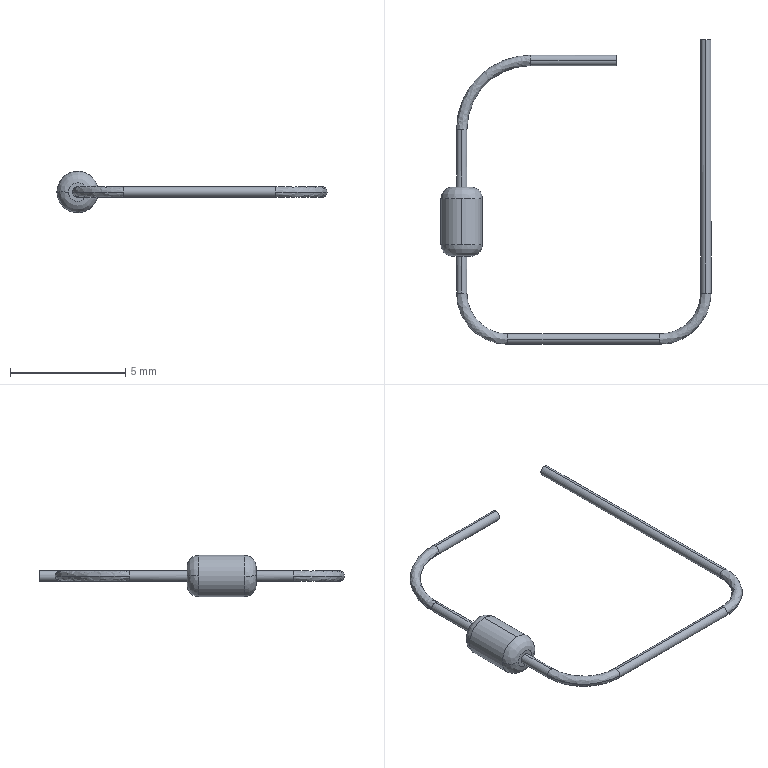Part | STEP file | TQ-DD-1105-THNTC Thermistor1010_デフォルト | 1 solid | 26 faces | box 11.725 x 13.225 x 1.8 mm | volume 12.894 mm3 | cylinder 12 | spline 10 | plane 4 | commonest cylinder face diameters 0.45 x10 1.8 x2
STEP:
#1=CARTESIAN_POINT('',(10.825,-3.1,0.));
#2=VERTEX_POINT('',#1);
#3=CARTESIAN_POINT('',(10.6,-3.1,-0.225));
#4=VERTEX_POINT('',#3);
#5=CARTESIAN_POINT('',(10.6,-3.1,0.));
#6=DIRECTION('',(0.,1.,0.));
#7=DIRECTION('',(0.,0.,1.));
#8=AXIS2_PLACEMENT_3D('',#5,#6,#7);
#9=CIRCLE('',#8,0.225);
#10=EDGE_CURVE('',#2,#4,#9,.T.);
#11=ORIENTED_EDGE('',*,*,#10,.T.);
#12=CARTESIAN_POINT('',(10.6,7.9,-0.225));
#13=VERTEX_POINT('',#12);
#14=CARTESIAN_POINT('',(10.6,2.4,-0.225));
#15=DIRECTION('',(0.,1.,0.));
#16=VECTOR('',#15,1000.);
#17=LINE('',#14,#16);
#18=EDGE_CURVE('',#4,#13,#17,.T.);
#19=ORIENTED_EDGE('',*,*,#18,.T.);
#20=CARTESIAN_POINT('',(10.6,7.9,0.225));
#21=VERTEX_POINT('',#20);
#22=CARTESIAN_POINT('',(10.6,7.9,0.));
#23=DIRECTION('',(0.,-1.,0.));
#24=DIRECTION('',(0.,0.,1.));
#25=AXIS2_PLACEMENT_3D('',#22,#23,#24);
#26=CIRCLE('',#25,0.225);
#27=EDGE_CURVE('',#13,#21,#26,.T.);
#28=ORIENTED_EDGE('',*,*,#27,.T.);
#29=CARTESIAN_POINT('',(10.6,-3.1,0.225));
#30=VERTEX_POINT('',#29);
#31=CARTESIAN_POINT('',(10.6,2.4,0.225));
#32=DIRECTION('',(0.,1.,0.));
#33=VECTOR('',#32,1000.);
#34=LINE('',#31,#33);
#35=EDGE_CURVE('',#30,#21,#34,.T.);
#36=ORIENTED_EDGE('',*,*,#35,.F.);
#37=CARTESIAN_POINT('',(10.6,-3.1,0.));
#38=DIRECTION('',(0.,1.,0.));
#39=DIRECTION('',(0.,0.,1.));
#40=AXIS2_PLACEMENT_3D('',#37,#38,#39);
#41=CIRCLE('',#40,0.225);
#42=EDGE_CURVE('',#30,#2,#41,.T.);
#43=ORIENTED_EDGE('',*,*,#42,.T.);
#44=EDGE_LOOP('',(#11,#19,#28,#36,#43));
#45=FACE_OUTER_BOUND('',#44,.T.);
#46=CARTESIAN_POINT('',(10.6,2.4,0.));
#47=DIRECTION('',(0.,1.,0.));
#48=DIRECTION('',(0.,0.,1.));
#49=AXIS2_PLACEMENT_3D('',#46,#47,#48);
#50=CYLINDRICAL_SURFACE('',#49,0.225);
#51=ADVANCED_FACE('',(#45),#50,.T.);
#52=CARTESIAN_POINT('',(8.6,-5.1,-0.225));
#53=VERTEX_POINT('',#52);
#54=CARTESIAN_POINT('',(8.6,-4.875,0.));
#55=VERTEX_POINT('',#54);
#56=CARTESIAN_POINT('',(8.6,-5.1,0.));
#57=DIRECTION('',(1.,0.,0.));
#58=DIRECTION('',(0.,-1.,0.));
#59=AXIS2_PLACEMENT_3D('',#56,#57,#58);
#60=CIRCLE('',#59,0.225);
#61=EDGE_CURVE('',#53,#55,#60,.T.);
#62=ORIENTED_EDGE('',*,*,#61,.T.);
#63=CARTESIAN_POINT('',(10.375,-3.1,0.));
#64=VERTEX_POINT('',#63);
#65=CARTESIAN_POINT('',(8.6,-3.1,0.));
#66=DIRECTION('',(0.,0.,1.));
#67=DIRECTION('',(0.,-1.,0.));
#68=AXIS2_PLACEMENT_3D('',#65,#66,#67);
#69=CIRCLE('',#68,1.775);
#70=EDGE_CURVE('',#55,#64,#69,.T.);
#71=ORIENTED_EDGE('',*,*,#70,.T.);
#72=CARTESIAN_POINT('',(10.6,-3.1,0.));
#73=DIRECTION('',(0.,1.,0.));
#74=DIRECTION('',(0.,0.,1.));
#75=AXIS2_PLACEMENT_3D('',#72,#73,#74);
#76=CIRCLE('',#75,0.225);
#77=EDGE_CURVE('',#4,#64,#76,.T.);
#78=ORIENTED_EDGE('',*,*,#77,.F.);
#79=ORIENTED_EDGE('',*,*,#10,.F.);
#80=CARTESIAN_POINT('',(8.6,-5.325,0.));
#81=VERTEX_POINT('',#80);
#82=CARTESIAN_POINT('',(8.6,-3.1,0.));
#83=DIRECTION('',(0.,0.,1.));
#84=DIRECTION('',(0.,-1.,0.));
#85=AXIS2_PLACEMENT_3D('',#82,#83,#84);
#86=CIRCLE('',#85,2.225);
#87=EDGE_CURVE('',#81,#2,#86,.T.);
#88=ORIENTED_EDGE('',*,*,#87,.F.);
#89=CARTESIAN_POINT('',(8.6,-5.1,0.));
#90=DIRECTION('',(1.,0.,0.));
#91=DIRECTION('',(0.,-1.,0.));
#92=AXIS2_PLACEMENT_3D('',#89,#90,#91);
#93=CIRCLE('',#92,0.225);
#94=EDGE_CURVE('',#81,#53,#93,.T.);
#95=ORIENTED_EDGE('',*,*,#94,.T.);
#96=EDGE_LOOP('',(#62,#71,#78,#79,#88,#95));
#97=FACE_OUTER_BOUND('',#96,.T.);
#98=CARTESIAN_POINT('',(8.6,-5.325,0.));
#99=CARTESIAN_POINT('',(9.903,-5.325,0.));
#100=CARTESIAN_POINT('',(10.825,-4.403,0.));
#101=CARTESIAN_POINT('',(10.825,-3.1,0.));
#102=CARTESIAN_POINT('',(8.6,-5.325,-0.45));
#103=CARTESIAN_POINT('',(9.903,-5.325,-0.45));
#104=CARTESIAN_POINT('',(10.825,-4.403,-0.45));
#105=CARTESIAN_POINT('',(10.825,-3.1,-0.45));
#106=CARTESIAN_POINT('',(8.6,-4.875,-0.45));
#107=CARTESIAN_POINT('',(9.64,-4.875,-0.45));
#108=CARTESIAN_POINT('',(10.375,-4.14,-0.45));
#109=CARTESIAN_POINT('',(10.375,-3.1,-0.45));
#110=CARTESIAN_POINT('',(8.6,-4.875,0.));
#111=CARTESIAN_POINT('',(9.64,-4.875,0.));
#112=CARTESIAN_POINT('',(10.375,-4.14,0.));
#113=CARTESIAN_POINT('',(10.375,-3.1,0.));
#114=(BOUNDED_SURFACE()B_SPLINE_SURFACE(3,3,((#98,#99,#100,#101),(#102,#103,#104,#105),(#106,#107,#108,#109),(#110,#111,#112,#113)),.UNSPECIFIED.,.F.,.F.,.F.)B_SPLINE_SURFACE_WITH_KNOTS((4,4),(4,4),(0.,1.),(0.,1.),.UNSPECIFIED.)GEOMETRIC_REPRESENTATION_ITEM()RATIONAL_B_SPLINE_SURFACE(((1.,0.8047,0.8047,1.),(0.3333,0.2682,0.2682,0.3333),(0.3333,0.2682,0.2682,0.3333),(1.,0.8047,0.8047,1.)))REPRESENTATION_ITEM('')SURFACE());
#115=ADVANCED_FACE('',(#97),#114,.T.);
#116=CARTESIAN_POINT('',(2.,-4.875,0.));
#117=VERTEX_POINT('',#116);
#118=CARTESIAN_POINT('',(2.,-5.1,0.225));
#119=VERTEX_POINT('',#118);
#120=CARTESIAN_POINT('',(2.,-5.1,0.));
#121=DIRECTION('',(1.,0.,0.));
#122=DIRECTION('',(0.,0.,-1.));
#123=AXIS2_PLACEMENT_3D('',#120,#121,#122);
#124=CIRCLE('',#123,0.225);
#125=EDGE_CURVE('',#117,#119,#124,.T.);
#126=ORIENTED_EDGE('',*,*,#125,.T.);
#127=CARTESIAN_POINT('',(8.6,-5.1,0.225));
#128=VERTEX_POINT('',#127);
#129=CARTESIAN_POINT('',(5.3,-5.1,0.225));
#130=DIRECTION('',(1.,0.,0.));
#131=VECTOR('',#130,1000.);
#132=LINE('',#129,#131);
#133=EDGE_CURVE('',#119,#128,#132,.T.);
#134=ORIENTED_EDGE('',*,*,#133,.T.);
#135=CARTESIAN_POINT('',(8.6,-5.1,0.));
#136=DIRECTION('',(1.,0.,0.));
#137=DIRECTION('',(0.,-1.,0.));
#138=AXIS2_PLACEMENT_3D('',#135,#136,#137);
#139=CIRCLE('',#138,0.225);
#140=EDGE_CURVE('',#55,#128,#139,.T.);
#141=ORIENTED_EDGE('',*,*,#140,.F.);
#142=ORIENTED_EDGE('',*,*,#61,.F.);
#143=CARTESIAN_POINT('',(2.,-5.1,-0.225));
#144=VERTEX_POINT('',#143);
#145=CARTESIAN_POINT('',(5.3,-5.1,-0.225));
#146=DIRECTION('',(1.,0.,0.));
#147=VECTOR('',#146,1000.);
#148=LINE('',#145,#147);
#149=EDGE_CURVE('',#144,#53,#148,.T.);
#150=ORIENTED_EDGE('',*,*,#149,.F.);
#151=CARTESIAN_POINT('',(2.,-5.1,0.));
#152=DIRECTION('',(1.,0.,0.));
#153=DIRECTION('',(0.,0.,-1.));
#154=AXIS2_PLACEMENT_3D('',#151,#152,#153);
#155=CIRCLE('',#154,0.225);
#156=EDGE_CURVE('',#144,#117,#155,.T.);
#157=ORIENTED_EDGE('',*,*,#156,.T.);
#158=EDGE_LOOP('',(#126,#134,#141,#142,#150,#157));
#159=FACE_OUTER_BOUND('',#158,.T.);
#160=CARTESIAN_POINT('',(5.3,-5.1,0.));
#161=DIRECTION('',(1.,0.,0.));
#162=DIRECTION('',(0.,0.,-1.));
#163=AXIS2_PLACEMENT_3D('',#160,#161,#162);
#164=CYLINDRICAL_SURFACE('',#163,0.225);
#165=ADVANCED_FACE('',(#159),#164,.T.);
#166=CARTESIAN_POINT('',(0.,-3.1,-0.225));
#167=VERTEX_POINT('',#166);
#168=CARTESIAN_POINT('',(0.225,-3.1,0.));
#169=VERTEX_POINT('',#168);
#170=CARTESIAN_POINT('',(0.,-3.1,0.));
#171=DIRECTION('',(0.,-1.,0.));
#172=DIRECTION('',(-1.,0.,0.));
#173=AXIS2_PLACEMENT_3D('',#170,#171,#172);
#174=CIRCLE('',#173,0.225);
#175=EDGE_CURVE('',#167,#169,#174,.T.);
#176=ORIENTED_EDGE('',*,*,#175,.T.);
#177=CARTESIAN_POINT('',(2.,-3.1,0.));
#178=DIRECTION('',(0.,0.,1.));
#179=DIRECTION('',(-1.,0.,0.));
#180=AXIS2_PLACEMENT_3D('',#177,#178,#179);
#181=CIRCLE('',#180,1.775);
#182=EDGE_CURVE('',#169,#117,#181,.T.);
#183=ORIENTED_EDGE('',*,*,#182,.T.);
#184=ORIENTED_EDGE('',*,*,#156,.F.);
#185=CARTESIAN_POINT('',(2.,-5.325,0.));
#186=VERTEX_POINT('',#185);
#187=CARTESIAN_POINT('',(2.,-5.1,0.));
#188=DIRECTION('',(1.,0.,0.));
#189=DIRECTION('',(0.,0.,-1.));
#190=AXIS2_PLACEMENT_3D('',#187,#188,#189);
#191=CIRCLE('',#190,0.225);
#192=EDGE_CURVE('',#186,#144,#191,.T.);
#193=ORIENTED_EDGE('',*,*,#192,.F.);
#194=CARTESIAN_POINT('',(-0.225,-3.1,0.));
#195=VERTEX_POINT('',#194);
#196=CARTESIAN_POINT('',(2.,-3.1,0.));
#197=DIRECTION('',(0.,0.,1.));
#198=DIRECTION('',(-1.,0.,0.));
#199=AXIS2_PLACEMENT_3D('',#196,#197,#198);
#200=CIRCLE('',#199,2.225);
#201=EDGE_CURVE('',#195,#186,#200,.T.);
#202=ORIENTED_EDGE('',*,*,#201,.F.);
#203=CARTESIAN_POINT('',(0.,-3.1,0.));
#204=DIRECTION('',(0.,-1.,0.));
#205=DIRECTION('',(-1.,0.,0.));
#206=AXIS2_PLACEMENT_3D('',#203,#204,#205);
#207=CIRCLE('',#206,0.225);
#208=EDGE_CURVE('',#195,#167,#207,.T.);
#209=ORIENTED_EDGE('',*,*,#208,.T.);
#210=EDGE_LOOP('',(#176,#183,#184,#193,#202,#209));
#211=FACE_OUTER_BOUND('',#210,.T.);
#212=CARTESIAN_POINT('',(-0.225,-3.1,0.));
#213=CARTESIAN_POINT('',(-0.225,-4.403,0.));
#214=CARTESIAN_POINT('',(0.6966,-5.325,0.));
#215=CARTESIAN_POINT('',(2.,-5.325,0.));
#216=CARTESIAN_POINT('',(-0.225,-3.1,-0.45));
#217=CARTESIAN_POINT('',(-0.225,-4.403,-0.45));
#218=CARTESIAN_POINT('',(0.6966,-5.325,-0.45));
#219=CARTESIAN_POINT('',(2.,-5.325,-0.45));
#220=CARTESIAN_POINT('',(0.225,-3.1,-0.45));
#221=CARTESIAN_POINT('',(0.225,-4.14,-0.45));
#222=CARTESIAN_POINT('',(0.9602,-4.875,-0.45));
#223=CARTESIAN_POINT('',(2.,-4.875,-0.45));
#224=CARTESIAN_POINT('',(0.225,-3.1,0.));
#225=CARTESIAN_POINT('',(0.225,-4.14,0.));
#226=CARTESIAN_POINT('',(0.9602,-4.875,0.));
#227=CARTESIAN_POINT('',(2.,-4.875,0.));
#228=(BOUNDED_SURFACE()B_SPLINE_SURFACE(3,3,((#212,#213,#214,#215),(#216,#217,#218,#219),(#220,#221,#222,#223),(#224,#225,#226,#227)),.UNSPECIFIED.,.F.,.F.,.F.)B_SPLINE_SURFACE_WITH_KNOTS((4,4),(4,4),(0.,1.),(0.,1.),.UNSPECIFIED.)GEOMETRIC_REPRESENTATION_ITEM()RATIONAL_B_SPLINE_SURFACE(((1.,0.8047,0.8047,1.),(0.3333,0.2682,0.2682,0.3333),(0.3333,0.2682,0.2682,0.3333),(1.,0.8047,0.8047,1.)))REPRESENTATION_ITEM('')SURFACE());
#229=ADVANCED_FACE('',(#211),#228,.T.);
#230=CARTESIAN_POINT('',(0.,-1.5,-0.225));
#231=VERTEX_POINT('',#230);
#232=CARTESIAN_POINT('',(0.,-1.5,0.225));
#233=VERTEX_POINT('',#232);
#234=CARTESIAN_POINT('',(0.,-1.5,0.));
#235=DIRECTION('',(0.,-1.,0.));
#236=DIRECTION('',(0.,0.,-1.));
#237=AXIS2_PLACEMENT_3D('',#234,#235,#236);
#238=CIRCLE('',#237,0.225);
#239=EDGE_CURVE('',#231,#233,#238,.T.);
#240=ORIENTED_EDGE('',*,*,#239,.T.);
#241=CARTESIAN_POINT('',(0.,-3.1,0.225));
#242=VERTEX_POINT('',#241);
#243=CARTESIAN_POINT('',(0.,-2.07,0.225));
#244=DIRECTION('',(0.,-1.,0.));
#245=VECTOR('',#244,1000.);
#246=LINE('',#243,#245);
#247=EDGE_CURVE('',#233,#242,#246,.T.);
#248=ORIENTED_EDGE('',*,*,#247,.T.);
#249=CARTESIAN_POINT('',(0.,-3.1,0.));
#250=DIRECTION('',(0.,-1.,0.));
#251=DIRECTION('',(-1.,0.,0.));
#252=AXIS2_PLACEMENT_3D('',#249,#250,#251);
#253=CIRCLE('',#252,0.225);
#254=EDGE_CURVE('',#169,#242,#253,.T.);
#255=ORIENTED_EDGE('',*,*,#254,.F.);
#256=ORIENTED_EDGE('',*,*,#175,.F.);
#257=CARTESIAN_POINT('',(0.,-2.07,-0.225));
#258=DIRECTION('',(0.,-1.,0.));
#259=VECTOR('',#258,1000.);
#260=LINE('',#257,#259);
#261=EDGE_CURVE('',#231,#167,#260,.T.);
#262=ORIENTED_EDGE('',*,*,#261,.F.);
#263=EDGE_LOOP('',(#240,#248,#255,#256,#262));
#264=FACE_OUTER_BOUND('',#263,.T.);
#265=CARTESIAN_POINT('',(0.,-2.07,0.));
#266=DIRECTION('',(0.,-1.,0.));
#267=DIRECTION('',(0.,0.,-1.));
#268=AXIS2_PLACEMENT_3D('',#265,#266,#267);
#269=CYLINDRICAL_SURFACE('',#268,0.225);
#270=ADVANCED_FACE('',(#264),#269,.T.);
#271=CARTESIAN_POINT('',(0.9,-1.,-0.000000339));
#272=VERTEX_POINT('',#271);
#273=CARTESIAN_POINT('',(0.,-1.,-0.9));
#274=VERTEX_POINT('',#273);
#275=CARTESIAN_POINT('',(0.,-1.,0.));
#276=DIRECTION('',(0.,1.,0.));
#277=DIRECTION('',(0.,0.,1.));
#278=AXIS2_PLACEMENT_3D('',#275,#276,#277);
#279=CIRCLE('',#278,0.9);
#280=EDGE_CURVE('',#272,#274,#279,.T.);
#281=ORIENTED_EDGE('',*,*,#280,.T.);
#282=CARTESIAN_POINT('',(0.,1.,-0.9));
#283=VERTEX_POINT('',#282);
#284=CARTESIAN_POINT('',(0.,0.,-0.9));
#285=DIRECTION('',(0.,1.,0.));
#286=VECTOR('',#285,1000.);
#287=LINE('',#284,#286);
#288=EDGE_CURVE('',#274,#283,#287,.T.);
#289=ORIENTED_EDGE('',*,*,#288,.T.);
#290=CARTESIAN_POINT('',(0.9,1.,-0.000000096));
#291=VERTEX_POINT('',#290);
#292=CARTESIAN_POINT('',(0.,1.,0.));
#293=DIRECTION('',(0.,-1.,0.));
#294=DIRECTION('',(0.,0.,1.));
#295=AXIS2_PLACEMENT_3D('',#292,#293,#294);
#296=CIRCLE('',#295,0.9);
#297=EDGE_CURVE('',#283,#291,#296,.T.);
#298=ORIENTED_EDGE('',*,*,#297,.T.);
#299=CARTESIAN_POINT('',(0.,1.,0.9));
#300=VERTEX_POINT('',#299);
#301=CARTESIAN_POINT('',(0.,1.,0.));
#302=DIRECTION('',(0.,-1.,0.));
#303=DIRECTION('',(0.,0.,1.));
#304=AXIS2_PLACEMENT_3D('',#301,#302,#303);
#305=CIRCLE('',#304,0.9);
#306=EDGE_CURVE('',#291,#300,#305,.T.);
#307=ORIENTED_EDGE('',*,*,#306,.T.);
#308=CARTESIAN_POINT('',(0.,-1.,0.9));
#309=VERTEX_POINT('',#308);
#310=CARTESIAN_POINT('',(0.,0.,0.9));
#311=DIRECTION('',(0.,1.,0.));
#312=VECTOR('',#311,1000.);
#313=LINE('',#310,#312);
#314=EDGE_CURVE('',#309,#300,#313,.T.);
#315=ORIENTED_EDGE('',*,*,#314,.F.);
#316=CARTESIAN_POINT('',(0.,-1.,0.));
#317=DIRECTION('',(0.,1.,0.));
#318=DIRECTION('',(-0.1409,0.,-0.99));
#319=AXIS2_PLACEMENT_3D('',#316,#317,#318);
#320=CIRCLE('',#319,0.9);
#321=EDGE_CURVE('',#309,#272,#320,.T.);
#322=ORIENTED_EDGE('',*,*,#321,.T.);
#323=EDGE_LOOP('',(#281,#289,#298,#307,#315,#322));
#324=FACE_OUTER_BOUND('',#323,.T.);
#325=CARTESIAN_POINT('',(0.,0.,0.));
#326=DIRECTION('',(0.,1.,0.));
#327=DIRECTION('',(0.,0.,1.));
#328=AXIS2_PLACEMENT_3D('',#325,#326,#327);
#329=CYLINDRICAL_SURFACE('',#328,0.9);
#330=ADVANCED_FACE('',(#324),#329,.T.);
#331=CARTESIAN_POINT('',(0.,1.5,-0.225));
#332=VERTEX_POINT('',#331);
#333=CARTESIAN_POINT('',(0.,1.5,0.225));
#334=VERTEX_POINT('',#333);
#335=CARTESIAN_POINT('',(0.,1.5,0.));
#336=DIRECTION('',(0.,-1.,0.));
#337=DIRECTION('',(0.,0.,1.));
#338=AXIS2_PLACEMENT_3D('',#335,#336,#337);
#339=CIRCLE('',#338,0.225);
#340=EDGE_CURVE('',#332,#334,#339,.T.);
#341=ORIENTED_EDGE('',*,*,#340,.F.);
#342=CARTESIAN_POINT('',(0.,4.,-0.225));
#343=VERTEX_POINT('',#342);
#344=CARTESIAN_POINT('',(0.,2.75,-0.225));
#345=DIRECTION('',(0.,1.,0.));
#346=VECTOR('',#345,1000.);
#347=LINE('',#344,#346);
#348=EDGE_CURVE('',#332,#343,#347,.T.);
#349=ORIENTED_EDGE('',*,*,#348,.T.);
#350=CARTESIAN_POINT('',(0.225,4.,0.));
#351=VERTEX_POINT('',#350);
#352=CARTESIAN_POINT('',(0.,4.,0.));
#353=DIRECTION('',(0.,-1.,0.));
#354=DIRECTION('',(0.,0.,1.));
#355=AXIS2_PLACEMENT_3D('',#352,#353,#354);
#356=CIRCLE('',#355,0.225);
#357=EDGE_CURVE('',#343,#351,#356,.T.);
#358=ORIENTED_EDGE('',*,*,#357,.T.);
#359=CARTESIAN_POINT('',(0.,4.,0.225));
#360=VERTEX_POINT('',#359);
#361=CARTESIAN_POINT('',(0.,4.,0.));
#362=DIRECTION('',(0.,-1.,0.));
#363=DIRECTION('',(0.,0.,1.));
#364=AXIS2_PLACEMENT_3D('',#361,#362,#363);
#365=CIRCLE('',#364,0.225);
#366=EDGE_CURVE('',#351,#360,#365,.T.);
#367=ORIENTED_EDGE('',*,*,#366,.T.);
#368=CARTESIAN_POINT('',(0.,2.75,0.225));
#369=DIRECTION('',(0.,1.,0.));
#370=VECTOR('',#369,1000.);
#371=LINE('',#368,#370);
#372=EDGE_CURVE('',#334,#360,#371,.T.);
#373=ORIENTED_EDGE('',*,*,#372,.F.);
#374=EDGE_LOOP('',(#341,#349,#358,#367,#373));
#375=FACE_OUTER_BOUND('',#374,.T.);
#376=CARTESIAN_POINT('',(0.,2.75,0.));
#377=DIRECTION('',(0.,1.,0.));
#378=DIRECTION('',(0.,0.,1.));
#379=AXIS2_PLACEMENT_3D('',#376,#377,#378);
#380=CYLINDRICAL_SURFACE('',#379,0.225);
#381=ADVANCED_FACE('',(#375),#380,.T.);
#382=CARTESIAN_POINT('',(3.,7.,-0.225));
#383=VERTEX_POINT('',#382);
#384=CARTESIAN_POINT('',(3.,6.775,0.));
#385=VERTEX_POINT('',#384);
#386=CARTESIAN_POINT('',(3.,7.,0.));
#387=DIRECTION('',(-1.,0.,0.));
#388=DIRECTION('',(0.,1.,0.));
#389=AXIS2_PLACEMENT_3D('',#386,#387,#388);
#390=CIRCLE('',#389,0.225);
#391=EDGE_CURVE('',#383,#385,#390,.T.);
#392=ORIENTED_EDGE('',*,*,#391,.T.);
#393=CARTESIAN_POINT('',(3.,4.,0.));
#394=DIRECTION('',(0.,0.,1.));
#395=DIRECTION('',(0.,1.,0.));
#396=AXIS2_PLACEMENT_3D('',#393,#394,#395);
#397=CIRCLE('',#396,2.775);
#398=EDGE_CURVE('',#385,#351,#397,.T.);
#399=ORIENTED_EDGE('',*,*,#398,.T.);
#400=ORIENTED_EDGE('',*,*,#357,.F.);
#401=CARTESIAN_POINT('',(-0.225,4.,0.));
#402=VERTEX_POINT('',#401);
#403=CARTESIAN_POINT('',(0.,4.,0.));
#404=DIRECTION('',(0.,-1.,0.));
#405=DIRECTION('',(0.,0.,1.));
#406=AXIS2_PLACEMENT_3D('',#403,#404,#405);
#407=CIRCLE('',#406,0.225);
#408=EDGE_CURVE('',#402,#343,#407,.T.);
#409=ORIENTED_EDGE('',*,*,#408,.F.);
#410=CARTESIAN_POINT('',(3.,7.225,0.));
#411=VERTEX_POINT('',#410);
#412=CARTESIAN_POINT('',(3.,4.,0.));
#413=DIRECTION('',(0.,0.,1.));
#414=DIRECTION('',(0.,1.,0.));
#415=AXIS2_PLACEMENT_3D('',#412,#413,#414);
#416=CIRCLE('',#415,3.225);
#417=EDGE_CURVE('',#411,#402,#416,.T.);
#418=ORIENTED_EDGE('',*,*,#417,.F.);
#419=CARTESIAN_POINT('',(3.,7.,0.));
#420=DIRECTION('',(-1.,0.,0.));
#421=DIRECTION('',(0.,1.,0.));
#422=AXIS2_PLACEMENT_3D('',#419,#420,#421);
#423=CIRCLE('',#422,0.225);
#424=EDGE_CURVE('',#411,#383,#423,.T.);
#425=ORIENTED_EDGE('',*,*,#424,.T.);
#426=EDGE_LOOP('',(#392,#399,#400,#409,#418,#425));
#427=FACE_OUTER_BOUND('',#426,.T.);
#428=CARTESIAN_POINT('',(3.,7.225,0.));
#429=CARTESIAN_POINT('',(1.111,7.225,0.));
#430=CARTESIAN_POINT('',(-0.225,5.889,0.));
#431=CARTESIAN_POINT('',(-0.225,4.,0.));
#432=CARTESIAN_POINT('',(3.,7.225,-0.45));
#433=CARTESIAN_POINT('',(1.111,7.225,-0.45));
#434=CARTESIAN_POINT('',(-0.225,5.889,-0.45));
#435=CARTESIAN_POINT('',(-0.225,4.,-0.45));
#436=CARTESIAN_POINT('',(3.,6.775,-0.45));
#437=CARTESIAN_POINT('',(1.374,6.775,-0.45));
#438=CARTESIAN_POINT('',(0.225,5.626,-0.45));
#439=CARTESIAN_POINT('',(0.225,4.,-0.45));
#440=CARTESIAN_POINT('',(3.,6.775,0.));
#441=CARTESIAN_POINT('',(1.374,6.775,0.));
#442=CARTESIAN_POINT('',(0.225,5.626,0.));
#443=CARTESIAN_POINT('',(0.225,4.,0.));
#444=(BOUNDED_SURFACE()B_SPLINE_SURFACE(3,3,((#428,#429,#430,#431),(#432,#433,#434,#435),(#436,#437,#438,#439),(#440,#441,#442,#443)),.UNSPECIFIED.,.F.,.F.,.F.)B_SPLINE_SURFACE_WITH_KNOTS((4,4),(4,4),(0.,1.),(0.,1.),.UNSPECIFIED.)GEOMETRIC_REPRESENTATION_ITEM()RATIONAL_B_SPLINE_SURFACE(((1.,0.8047,0.8047,1.),(0.3333,0.2682,0.2682,0.3333),(0.3333,0.2682,0.2682,0.3333),(1.,0.8047,0.8047,1.)))REPRESENTATION_ITEM('')SURFACE());
#445=ADVANCED_FACE('',(#427),#444,.T.);
#446=CARTESIAN_POINT('',(3.,7.,0.225));
#447=VERTEX_POINT('',#446);
#448=CARTESIAN_POINT('',(3.,7.,0.));
#449=DIRECTION('',(-1.,0.,0.));
#450=DIRECTION('',(0.,1.,0.));
#451=AXIS2_PLACEMENT_3D('',#448,#449,#450);
#452=CIRCLE('',#451,0.225);
#453=EDGE_CURVE('',#447,#411,#452,.T.);
#454=ORIENTED_EDGE('',*,*,#453,.F.);
#455=CARTESIAN_POINT('',(6.717,7.,0.225));
#456=VERTEX_POINT('',#455);
#457=CARTESIAN_POINT('',(4.858,7.,0.225));
#458=DIRECTION('',(1.,0.,0.));
#459=VECTOR('',#458,1000.);
#460=LINE('',#457,#459);
#461=EDGE_CURVE('',#447,#456,#460,.T.);
#462=ORIENTED_EDGE('',*,*,#461,.T.);
#463=CARTESIAN_POINT('',(6.717,7.,-0.225));
#464=VERTEX_POINT('',#463);
#465=CARTESIAN_POINT('',(6.717,7.,0.));
#466=DIRECTION('',(-1.,0.,0.));
#467=DIRECTION('',(0.,0.,-1.));
#468=AXIS2_PLACEMENT_3D('',#465,#466,#467);
#469=CIRCLE('',#468,0.225);
#470=EDGE_CURVE('',#456,#464,#469,.T.);
#471=ORIENTED_EDGE('',*,*,#470,.T.);
#472=CARTESIAN_POINT('',(4.858,7.,-0.225));
#473=DIRECTION('',(1.,0.,0.));
#474=VECTOR('',#473,1000.);
#475=LINE('',#472,#474);
#476=EDGE_CURVE('',#383,#464,#475,.T.);
#477=ORIENTED_EDGE('',*,*,#476,.F.);
#478=ORIENTED_EDGE('',*,*,#424,.F.);
#479=EDGE_LOOP('',(#454,#462,#471,#477,#478));
#480=FACE_OUTER_BOUND('',#479,.T.);
#481=CARTESIAN_POINT('',(4.858,7.,0.));
#482=DIRECTION('',(1.,0.,0.));
#483=DIRECTION('',(0.,0.,-1.));
#484=AXIS2_PLACEMENT_3D('',#481,#482,#483);
#485=CYLINDRICAL_SURFACE('',#484,0.225);
#486=ADVANCED_FACE('',(#480),#485,.T.);
#487=ORIENTED_EDGE('',*,*,#18,.F.);
#488=ORIENTED_EDGE('',*,*,#77,.T.);
#489=CARTESIAN_POINT('',(10.6,-3.1,0.));
#490=DIRECTION('',(0.,1.,0.));
#491=DIRECTION('',(0.,0.,1.));
#492=AXIS2_PLACEMENT_3D('',#489,#490,#491);
#493=CIRCLE('',#492,0.225);
#494=EDGE_CURVE('',#64,#30,#493,.T.);
#495=ORIENTED_EDGE('',*,*,#494,.T.);
#496=ORIENTED_EDGE('',*,*,#35,.T.);
#497=CARTESIAN_POINT('',(10.6,7.9,0.));
#498=DIRECTION('',(0.,-1.,0.));
#499=DIRECTION('',(0.,0.,1.));
#500=AXIS2_PLACEMENT_3D('',#497,#498,#499);
#501=CIRCLE('',#500,0.225);
#502=EDGE_CURVE('',#21,#13,#501,.T.);
#503=ORIENTED_EDGE('',*,*,#502,.T.);
#504=EDGE_LOOP('',(#487,#488,#495,#496,#503));
#505=FACE_OUTER_BOUND('',#504,.T.);
#506=CARTESIAN_POINT('',(10.6,2.4,0.));
#507=DIRECTION('',(0.,1.,0.));
#508=DIRECTION('',(0.,0.,1.));
#509=AXIS2_PLACEMENT_3D('',#506,#507,#508);
#510=CYLINDRICAL_SURFACE('',#509,0.225);
#511=ADVANCED_FACE('',(#505),#510,.T.);
#512=ORIENTED_EDGE('',*,*,#502,.F.);
#513=ORIENTED_EDGE('',*,*,#27,.F.);
#514=EDGE_LOOP('',(#512,#513));
#515=FACE_OUTER_BOUND('',#514,.T.);
#516=CARTESIAN_POINT('',(10.6,7.9,0.));
#517=DIRECTION('',(0.,1.,0.));
#518=DIRECTION('',(0.,0.,1.));
#519=AXIS2_PLACEMENT_3D('',#516,#517,#518);
#520=PLANE('',#519);
#521=ADVANCED_FACE('',(#515),#520,.T.);
#522=ORIENTED_EDGE('',*,*,#70,.F.);
#523=ORIENTED_EDGE('',*,*,#140,.T.);
#524=CARTESIAN_POINT('',(8.6,-5.1,0.));
#525=DIRECTION('',(1.,0.,0.));
#526=DIRECTION('',(0.,-1.,0.));
#527=AXIS2_PLACEMENT_3D('',#524,#525,#526);
#528=CIRCLE('',#527,0.225);
#529=EDGE_CURVE('',#128,#81,#528,.T.);
#530=ORIENTED_EDGE('',*,*,#529,.T.);
#531=ORIENTED_EDGE('',*,*,#87,.T.);
#532=ORIENTED_EDGE('',*,*,#42,.F.);
#533=ORIENTED_EDGE('',*,*,#494,.F.);
#534=EDGE_LOOP('',(#522,#523,#530,#531,#532,#533));
#535=FACE_OUTER_BOUND('',#534,.T.);
#536=CARTESIAN_POINT('',(8.6,-4.875,0.));
#537=CARTESIAN_POINT('',(9.64,-4.875,0.));
#538=CARTESIAN_POINT('',(10.375,-4.14,0.));
#539=CARTESIAN_POINT('',(10.375,-3.1,0.));
#540=CARTESIAN_POINT('',(8.6,-4.875,0.45));
#541=CARTESIAN_POINT('',(9.64,-4.875,0.45));
#542=CARTESIAN_POINT('',(10.375,-4.14,0.45));
#543=CARTESIAN_POINT('',(10.375,-3.1,0.45));
#544=CARTESIAN_POINT('',(8.6,-5.325,0.45));
#545=CARTESIAN_POINT('',(9.903,-5.325,0.45));
#546=CARTESIAN_POINT('',(10.825,-4.403,0.45));
#547=CARTESIAN_POINT('',(10.825,-3.1,0.45));
#548=CARTESIAN_POINT('',(8.6,-5.325,0.));
#549=CARTESIAN_POINT('',(9.903,-5.325,0.));
#550=CARTESIAN_POINT('',(10.825,-4.403,0.));
#551=CARTESIAN_POINT('',(10.825,-3.1,0.));
#552=(BOUNDED_SURFACE()B_SPLINE_SURFACE(3,3,((#536,#537,#538,#539),(#540,#541,#542,#543),(#544,#545,#546,#547),(#548,#549,#550,#551)),.UNSPECIFIED.,.F.,.F.,.F.)B_SPLINE_SURFACE_WITH_KNOTS((4,4),(4,4),(0.,1.),(0.,1.),.UNSPECIFIED.)GEOMETRIC_REPRESENTATION_ITEM()RATIONAL_B_SPLINE_SURFACE(((1.,0.8047,0.8047,1.),(0.3333,0.2682,0.2682,0.3333),(0.3333,0.2682,0.2682,0.3333),(1.,0.8047,0.8047,1.)))REPRESENTATION_ITEM('')SURFACE());
#553=ADVANCED_FACE('',(#535),#552,.T.);
#554=ORIENTED_EDGE('',*,*,#133,.F.);
#555=CARTESIAN_POINT('',(2.,-5.1,0.));
#556=DIRECTION('',(1.,0.,0.));
#557=DIRECTION('',(0.,0.,-1.));
#558=AXIS2_PLACEMENT_3D('',#555,#556,#557);
#559=CIRCLE('',#558,0.225);
#560=EDGE_CURVE('',#119,#186,#559,.T.);
#561=ORIENTED_EDGE('',*,*,#560,.T.);
#562=ORIENTED_EDGE('',*,*,#192,.T.);
#563=ORIENTED_EDGE('',*,*,#149,.T.);
#564=ORIENTED_EDGE('',*,*,#94,.F.);
#565=ORIENTED_EDGE('',*,*,#529,.F.);
#566=EDGE_LOOP('',(#554,#561,#562,#563,#564,#565));
#567=FACE_OUTER_BOUND('',#566,.T.);
#568=CARTESIAN_POINT('',(5.3,-5.1,0.));
#569=DIRECTION('',(1.,0.,0.));
#570=DIRECTION('',(0.,0.,-1.));
#571=AXIS2_PLACEMENT_3D('',#568,#569,#570);
#572=CYLINDRICAL_SURFACE('',#571,0.225);
#573=ADVANCED_FACE('',(#567),#572,.T.);
#574=ORIENTED_EDGE('',*,*,#182,.F.);
#575=ORIENTED_EDGE('',*,*,#254,.T.);
#576=CARTESIAN_POINT('',(0.,-3.1,0.));
#577=DIRECTION('',(0.,-1.,0.));
#578=DIRECTION('',(-1.,0.,0.));
#579=AXIS2_PLACEMENT_3D('',#576,#577,#578);
#580=CIRCLE('',#579,0.225);
#581=EDGE_CURVE('',#242,#195,#580,.T.);
#582=ORIENTED_EDGE('',*,*,#581,.T.);
#583=ORIENTED_EDGE('',*,*,#201,.T.);
#584=ORIENTED_EDGE('',*,*,#560,.F.);
#585=ORIENTED_EDGE('',*,*,#125,.F.);
#586=EDGE_LOOP('',(#574,#575,#582,#583,#584,#585));
#587=FACE_OUTER_BOUND('',#586,.T.);
#588=CARTESIAN_POINT('',(0.225,-3.1,0.));
#589=CARTESIAN_POINT('',(0.225,-4.14,0.));
#590=CARTESIAN_POINT('',(0.9602,-4.875,0.));
#591=CARTESIAN_POINT('',(2.,-4.875,0.));
#592=CARTESIAN_POINT('',(0.225,-3.1,0.45));
#593=CARTESIAN_POINT('',(0.225,-4.14,0.45));
#594=CARTESIAN_POINT('',(0.9602,-4.875,0.45));
#595=CARTESIAN_POINT('',(2.,-4.875,0.45));
#596=CARTESIAN_POINT('',(-0.225,-3.1,0.45));
#597=CARTESIAN_POINT('',(-0.225,-4.403,0.45));
#598=CARTESIAN_POINT('',(0.6966,-5.325,0.45));
#599=CARTESIAN_POINT('',(2.,-5.325,0.45));
#600=CARTESIAN_POINT('',(-0.225,-3.1,0.));
#601=CARTESIAN_POINT('',(-0.225,-4.403,0.));
#602=CARTESIAN_POINT('',(0.6966,-5.325,0.));
#603=CARTESIAN_POINT('',(2.,-5.325,0.));
#604=(BOUNDED_SURFACE()B_SPLINE_SURFACE(3,3,((#588,#589,#590,#591),(#592,#593,#594,#595),(#596,#597,#598,#599),(#600,#601,#602,#603)),.UNSPECIFIED.,.F.,.F.,.F.)B_SPLINE_SURFACE_WITH_KNOTS((4,4),(4,4),(0.,1.),(0.,1.),.UNSPECIFIED.)GEOMETRIC_REPRESENTATION_ITEM()RATIONAL_B_SPLINE_SURFACE(((1.,0.8047,0.8047,1.),(0.3333,0.2682,0.2682,0.3333),(0.3333,0.2682,0.2682,0.3333),(1.,0.8047,0.8047,1.)))REPRESENTATION_ITEM('')SURFACE());
#605=ADVANCED_FACE('',(#587),#604,.T.);
#606=ORIENTED_EDGE('',*,*,#247,.F.);
#607=CARTESIAN_POINT('',(0.,-1.5,0.));
#608=DIRECTION('',(0.,-1.,0.));
#609=DIRECTION('',(0.,0.,-1.));
#610=AXIS2_PLACEMENT_3D('',#607,#608,#609);
#611=CIRCLE('',#610,0.225);
#612=EDGE_CURVE('',#233,#231,#611,.T.);
#613=ORIENTED_EDGE('',*,*,#612,.T.);
#614=ORIENTED_EDGE('',*,*,#261,.T.);
#615=ORIENTED_EDGE('',*,*,#208,.F.);
#616=ORIENTED_EDGE('',*,*,#581,.F.);
#617=EDGE_LOOP('',(#606,#613,#614,#615,#616));
#618=FACE_OUTER_BOUND('',#617,.T.);
#619=CARTESIAN_POINT('',(0.,-2.07,0.));
#620=DIRECTION('',(0.,-1.,0.));
#621=DIRECTION('',(0.,0.,-1.));
#622=AXIS2_PLACEMENT_3D('',#619,#620,#621);
#623=CYLINDRICAL_SURFACE('',#622,0.225);
#624=ADVANCED_FACE('',(#618),#623,.T.);
#625=ORIENTED_EDGE('',*,*,#239,.F.);
#626=ORIENTED_EDGE('',*,*,#612,.F.);
#627=EDGE_LOOP('',(#625,#626));
#628=FACE_BOUND('',#627,.T.);
#629=CARTESIAN_POINT('',(-0.4,-1.5,0.));
#630=VERTEX_POINT('',#629);
#631=CARTESIAN_POINT('',(0.4,-1.5,-0.000000314));
#632=VERTEX_POINT('',#631);
#633=CARTESIAN_POINT('',(-0.4,-1.5,0.));
#634=CARTESIAN_POINT('',(-0.3999,-1.5,-0.02569));
#635=CARTESIAN_POINT('',(-0.3964,-1.5,-0.06337));
#636=CARTESIAN_POINT('',(-0.3876,-1.5,-0.09974));
#637=CARTESIAN_POINT('',(-0.3806,-1.5,-0.1237));
#638=CARTESIAN_POINT('',(-0.377,-1.5,-0.1343));
#639=CARTESIAN_POINT('',(-0.3514,-1.5,-0.1989));
#640=CARTESIAN_POINT('',(-0.3222,-1.5,-0.2436));
#641=CARTESIAN_POINT('',(-0.2632,-1.5,-0.3025));
#642=CARTESIAN_POINT('',(-0.242,-1.5,-0.3197));
#643=CARTESIAN_POINT('',(-0.1968,-1.5,-0.3494));
#644=CARTESIAN_POINT('',(-0.1711,-1.5,-0.3625));
#645=CARTESIAN_POINT('',(-0.0996,-1.5,-0.3907));
#646=CARTESIAN_POINT('',(-0.05121,-1.5,-0.4001));
#647=CARTESIAN_POINT('',(0.02561,-1.5,-0.4));
#648=CARTESIAN_POINT('',(0.06322,-1.5,-0.3964));
#649=CARTESIAN_POINT('',(0.09963,-1.5,-0.3877));
#650=CARTESIAN_POINT('',(0.1236,-1.5,-0.3807));
#651=CARTESIAN_POINT('',(0.1343,-1.5,-0.377));
#652=CARTESIAN_POINT('',(0.1989,-1.5,-0.3514));
#653=CARTESIAN_POINT('',(0.2436,-1.5,-0.3222));
#654=CARTESIAN_POINT('',(0.3025,-1.5,-0.2632));
#655=CARTESIAN_POINT('',(0.3197,-1.5,-0.242));
#656=CARTESIAN_POINT('',(0.3494,-1.5,-0.1968));
#657=CARTESIAN_POINT('',(0.3626,-1.5,-0.1708));
#658=CARTESIAN_POINT('',(0.3905,-1.5,-0.1001));
#659=CARTESIAN_POINT('',(0.3999,-1.5,-0.05103));
#660=CARTESIAN_POINT('',(0.4,-1.5,-0.000000314));
#661=B_SPLINE_CURVE_WITH_KNOTS('',3,(#633,#634,#635,#636,#637,#638,#639,#640,#641,#642,#643,#644,#645,#646,#647,#648,#649,#650,#651,#652,#653,#654,#655,#656,#657,#658,#659,#660),.UNSPECIFIED.,.F.,.F.,(4,1,2,2,2,2,2,2,1,2,2,2,2,2,4),(0.,0.0625,0.09375,0.125,0.25,0.3125,0.375,0.5,0.5625,0.5938,0.625,0.75,0.8125,0.875,1.),.UNSPECIFIED.);
#662=EDGE_CURVE('',#630,#632,#661,.T.);
#663=ORIENTED_EDGE('',*,*,#662,.T.);
#664=CARTESIAN_POINT('',(-0.4,-1.5,0.));
#665=CARTESIAN_POINT('',(-0.4,-1.5,0.2343));
#666=CARTESIAN_POINT('',(-0.2343,-1.5,0.4));
#667=CARTESIAN_POINT('',(0.000000188,-1.5,0.4));
#668=CARTESIAN_POINT('',(0.2343,-1.5,0.4));
#669=CARTESIAN_POINT('',(0.4,-1.5,0.2343));
#670=CARTESIAN_POINT('',(0.4,-1.5,-0.000000314));
#671=(BOUNDED_CURVE()B_SPLINE_CURVE(3,(#664,#665,#666,#667,#668,#669,#670),.UNSPECIFIED.,.F.,.T.)B_SPLINE_CURVE_WITH_KNOTS((4,3,4),(0.,0.5,1.),.UNSPECIFIED.)CURVE()GEOMETRIC_REPRESENTATION_ITEM()RATIONAL_B_SPLINE_CURVE((1.,0.8047,0.8047,1.,0.8047,0.8047,1.))REPRESENTATION_ITEM(''));
#672=EDGE_CURVE('',#630,#632,#671,.T.);
#673=ORIENTED_EDGE('',*,*,#672,.F.);
#674=EDGE_LOOP('',(#663,#673));
#675=FACE_OUTER_BOUND('',#674,.T.);
#676=CARTESIAN_POINT('',(0.,-1.5,0.));
#677=DIRECTION('',(0.,1.,0.));
#678=DIRECTION('',(0.,0.,1.));
#679=AXIS2_PLACEMENT_3D('',#676,#677,#678);
#680=PLANE('',#679);
#681=ADVANCED_FACE('',(#628,#675),#680,.F.);
#682=ORIENTED_EDGE('',*,*,#672,.T.);
#683=CARTESIAN_POINT('',(0.4,-1.5,-0.000000314));
#684=CARTESIAN_POINT('',(0.5963,-1.5,0.));
#685=CARTESIAN_POINT('',(0.7952,-1.395,0.));
#686=CARTESIAN_POINT('',(0.9,-1.196,0.));
#687=CARTESIAN_POINT('',(0.9,-1.,-0.000000339));
#688=B_SPLINE_CURVE_WITH_KNOTS('',4,(#683,#684,#685,#686,#687),.UNSPECIFIED.,.F.,.F.,(5,5),(0.,1.),.UNSPECIFIED.);
#689=EDGE_CURVE('',#632,#272,#688,.T.);
#690=ORIENTED_EDGE('',*,*,#689,.T.);
#691=ORIENTED_EDGE('',*,*,#321,.F.);
#692=CARTESIAN_POINT('',(-0.9,-1.,0.));
#693=VERTEX_POINT('',#692);
#694=CARTESIAN_POINT('',(0.,-1.,0.));
#695=DIRECTION('',(0.,1.,0.));
#696=DIRECTION('',(-0.1409,0.,-0.99));
#697=AXIS2_PLACEMENT_3D('',#694,#695,#696);
#698=CIRCLE('',#697,0.9);
#699=EDGE_CURVE('',#693,#309,#698,.T.);
#700=ORIENTED_EDGE('',*,*,#699,.F.);
#701=CARTESIAN_POINT('',(-0.9,-1.,0.));
#702=CARTESIAN_POINT('',(-0.9,-1.196,0.));
#703=CARTESIAN_POINT('',(-0.7952,-1.395,0.));
#704=CARTESIAN_POINT('',(-0.5963,-1.5,0.));
#705=CARTESIAN_POINT('',(-0.4,-1.5,0.));
#706=B_SPLINE_CURVE_WITH_KNOTS('',4,(#701,#702,#703,#704,#705),.UNSPECIFIED.,.F.,.F.,(5,5),(0.,1.),.UNSPECIFIED.);
#707=EDGE_CURVE('',#693,#630,#706,.T.);
#708=ORIENTED_EDGE('',*,*,#707,.T.);
#709=EDGE_LOOP('',(#682,#690,#691,#700,#708));
#710=FACE_OUTER_BOUND('',#709,.T.);
#711=CARTESIAN_POINT('',(-0.4,-1.5,0.));
#712=CARTESIAN_POINT('',(-0.4,-1.5,0.8));
#713=CARTESIAN_POINT('',(0.4,-1.5,0.8));
#714=CARTESIAN_POINT('',(0.4,-1.5,0.));
#715=CARTESIAN_POINT('',(-0.5963,-1.5,0.));
#716=CARTESIAN_POINT('',(-0.5963,-1.5,1.193));
#717=CARTESIAN_POINT('',(0.5963,-1.5,1.193));
#718=CARTESIAN_POINT('',(0.5963,-1.5,0.));
#719=CARTESIAN_POINT('',(-0.7952,-1.395,0.));
#720=CARTESIAN_POINT('',(-0.7952,-1.395,1.59));
#721=CARTESIAN_POINT('',(0.7952,-1.395,1.59));
#722=CARTESIAN_POINT('',(0.7952,-1.395,0.));
#723=CARTESIAN_POINT('',(-0.9,-1.196,0.));
#724=CARTESIAN_POINT('',(-0.9,-1.196,1.8));
#725=CARTESIAN_POINT('',(0.9,-1.196,1.8));
#726=CARTESIAN_POINT('',(0.9,-1.196,0.));
#727=CARTESIAN_POINT('',(-0.9,-1.,0.));
#728=CARTESIAN_POINT('',(-0.9,-1.,1.8));
#729=CARTESIAN_POINT('',(0.9,-1.,1.8));
#730=CARTESIAN_POINT('',(0.9,-1.,0.));
#731=(BOUNDED_SURFACE()B_SPLINE_SURFACE(4,3,((#711,#712,#713,#714),(#715,#716,#717,#718),(#719,#720,#721,#722),(#723,#724,#725,#726),(#727,#728,#729,#730)),.UNSPECIFIED.,.F.,.F.,.F.)B_SPLINE_SURFACE_WITH_KNOTS((5,5),(4,4),(-0.7854,0.),(0.,1.),.UNSPECIFIED.)GEOMETRIC_REPRESENTATION_ITEM()RATIONAL_B_SPLINE_SURFACE(((1.,0.3333,0.3333,1.),(1.,0.3333,0.3333,1.),(1.,0.3333,0.3333,1.),(1.,0.3333,0.3333,1.),(1.,0.3333,0.3333,1.)))REPRESENTATION_ITEM('')SURFACE());
#732=ADVANCED_FACE('',(#710),#731,.F.);
#733=ORIENTED_EDGE('',*,*,#288,.F.);
#734=CARTESIAN_POINT('',(0.,-1.,0.));
#735=DIRECTION('',(0.,1.,0.));
#736=DIRECTION('',(0.,0.,1.));
#737=AXIS2_PLACEMENT_3D('',#734,#735,#736);
#738=CIRCLE('',#737,0.9);
#739=EDGE_CURVE('',#274,#693,#738,.T.);
#740=ORIENTED_EDGE('',*,*,#739,.T.);
#741=ORIENTED_EDGE('',*,*,#699,.T.);
#742=ORIENTED_EDGE('',*,*,#314,.T.);
#743=CARTESIAN_POINT('',(-0.9,1.,0.));
#744=VERTEX_POINT('',#743);
#745=CARTESIAN_POINT('',(0.,1.,0.));
#746=DIRECTION('',(0.,-1.,0.));
#747=DIRECTION('',(0.,0.,1.));
#748=AXIS2_PLACEMENT_3D('',#745,#746,#747);
#749=CIRCLE('',#748,0.9);
#750=EDGE_CURVE('',#300,#744,#749,.T.);
#751=ORIENTED_EDGE('',*,*,#750,.T.);
#752=CARTESIAN_POINT('',(0.,1.,0.));
#753=DIRECTION('',(0.,-1.,0.));
#754=DIRECTION('',(0.,0.,1.));
#755=AXIS2_PLACEMENT_3D('',#752,#753,#754);
#756=CIRCLE('',#755,0.9);
#757=EDGE_CURVE('',#744,#283,#756,.T.);
#758=ORIENTED_EDGE('',*,*,#757,.T.);
#759=EDGE_LOOP('',(#733,#740,#741,#742,#751,#758));
#760=FACE_OUTER_BOUND('',#759,.T.);
#761=CARTESIAN_POINT('',(0.,0.,0.));
#762=DIRECTION('',(0.,1.,0.));
#763=DIRECTION('',(0.,0.,1.));
#764=AXIS2_PLACEMENT_3D('',#761,#762,#763);
#765=CYLINDRICAL_SURFACE('',#764,0.9);
#766=ADVANCED_FACE('',(#760),#765,.T.);
#767=ORIENTED_EDGE('',*,*,#306,.F.);
#768=CARTESIAN_POINT('',(0.4,1.5,-0.000000143));
#769=VERTEX_POINT('',#768);
#770=CARTESIAN_POINT('',(0.4,1.5,-0.000000143));
#771=CARTESIAN_POINT('',(0.5963,1.5,0.));
#772=CARTESIAN_POINT('',(0.7952,1.395,0.));
#773=CARTESIAN_POINT('',(0.9,1.196,0.));
#774=CARTESIAN_POINT('',(0.9,1.,-0.000000096));
#775=B_SPLINE_CURVE_WITH_KNOTS('',4,(#770,#771,#772,#773,#774),.UNSPECIFIED.,.F.,.F.,(5,5),(0.,1.),.UNSPECIFIED.);
#776=EDGE_CURVE('',#769,#291,#775,.T.);
#777=ORIENTED_EDGE('',*,*,#776,.F.);
#778=CARTESIAN_POINT('',(-0.4,1.5,0.));
#779=VERTEX_POINT('',#778);
#780=CARTESIAN_POINT('',(-0.4,1.5,0.));
#781=CARTESIAN_POINT('',(-0.3999,1.5,0.0528));
#782=CARTESIAN_POINT('',(-0.3903,1.5,0.1023));
#783=CARTESIAN_POINT('',(-0.3598,1.5,0.1769));
#784=CARTESIAN_POINT('',(-0.3474,1.5,0.2003));
#785=CARTESIAN_POINT('',(-0.3179,1.5,0.2444));
#786=CARTESIAN_POINT('',(-0.2998,1.5,0.266));
#787=CARTESIAN_POINT('',(-0.245,1.5,0.3204));
#788=CARTESIAN_POINT('',(-0.2036,1.5,0.3483));
#789=CARTESIAN_POINT('',(-0.1054,1.5,0.3896));
#790=CARTESIAN_POINT('',(-0.05324,1.5,0.3999));
#791=CARTESIAN_POINT('',(0.02662,1.5,0.4));
#792=CARTESIAN_POINT('',(0.05281,1.5,0.3975));
#793=CARTESIAN_POINT('',(0.1043,1.5,0.3871));
#794=CARTESIAN_POINT('',(0.1308,1.5,0.3789));
#795=CARTESIAN_POINT('',(0.2021,1.5,0.3491));
#796=CARTESIAN_POINT('',(0.2433,1.5,0.3219));
#797=CARTESIAN_POINT('',(0.3007,1.5,0.2652));
#798=CARTESIAN_POINT('',(0.3176,1.5,0.2448));
#799=CARTESIAN_POINT('',(0.3471,1.5,0.2007));
#800=CARTESIAN_POINT('',(0.3601,1.5,0.1761));
#801=CARTESIAN_POINT('',(0.3899,1.5,0.1038));
#802=CARTESIAN_POINT('',(0.3999,1.5,0.05316));
#803=CARTESIAN_POINT('',(0.4,1.5,-0.000000143));
#804=B_SPLINE_CURVE_WITH_KNOTS('',3,(#780,#781,#782,#783,#784,#785,#786,#787,#788,#789,#790,#791,#792,#793,#794,#795,#796,#797,#798,#799,#800,#801,#802,#803),.UNSPECIFIED.,.F.,.F.,(4,2,2,2,2,2,2,2,2,2,2,4),(0.,0.125,0.1875,0.25,0.375,0.5,0.5625,0.625,0.75,0.8125,0.875,1.),.UNSPECIFIED.);
#805=EDGE_CURVE('',#779,#769,#804,.T.);
#806=ORIENTED_EDGE('',*,*,#805,.F.);
#807=CARTESIAN_POINT('',(-0.9,1.,0.));
#808=CARTESIAN_POINT('',(-0.9,1.196,0.));
#809=CARTESIAN_POINT('',(-0.7952,1.395,0.));
#810=CARTESIAN_POINT('',(-0.5963,1.5,0.));
#811=CARTESIAN_POINT('',(-0.4,1.5,0.));
#812=B_SPLINE_CURVE_WITH_KNOTS('',4,(#807,#808,#809,#810,#811),.UNSPECIFIED.,.F.,.F.,(5,5),(0.,1.),.UNSPECIFIED.);
#813=EDGE_CURVE('',#744,#779,#812,.T.);
#814=ORIENTED_EDGE('',*,*,#813,.F.);
#815=ORIENTED_EDGE('',*,*,#750,.F.);
#816=EDGE_LOOP('',(#767,#777,#806,#814,#815));
#817=FACE_OUTER_BOUND('',#816,.T.);
#818=CARTESIAN_POINT('',(-0.9,1.,0.));
#819=CARTESIAN_POINT('',(-0.9,1.,0.5272));
#820=CARTESIAN_POINT('',(-0.5272,1.,0.9));
#821=CARTESIAN_POINT('',(0.000000241,1.,0.9));
#822=CARTESIAN_POINT('',(0.5272,1.,0.9));
#823=CARTESIAN_POINT('',(0.9,1.,0.5272));
#824=CARTESIAN_POINT('',(0.9,1.,-0.000000481));
#825=CARTESIAN_POINT('',(-0.9,1.196,0.));
#826=CARTESIAN_POINT('',(-0.9,1.196,0.5272));
#827=CARTESIAN_POINT('',(-0.5272,1.196,0.9));
#828=CARTESIAN_POINT('',(0.000000241,1.196,0.9));
#829=CARTESIAN_POINT('',(0.5272,1.196,0.9));
#830=CARTESIAN_POINT('',(0.9,1.196,0.5272));
#831=CARTESIAN_POINT('',(0.9,1.196,-0.000000481));
#832=CARTESIAN_POINT('',(-0.7952,1.395,0.));
#833=CARTESIAN_POINT('',(-0.7952,1.395,0.4658));
#834=CARTESIAN_POINT('',(-0.4658,1.395,0.7952));
#835=CARTESIAN_POINT('',(0.000000213,1.395,0.7952));
#836=CARTESIAN_POINT('',(0.4658,1.395,0.7952));
#837=CARTESIAN_POINT('',(0.7952,1.395,0.4658));
#838=CARTESIAN_POINT('',(0.7952,1.395,-0.000000425));
#839=CARTESIAN_POINT('',(-0.5963,1.5,0.));
#840=CARTESIAN_POINT('',(-0.5963,1.5,0.3493));
#841=CARTESIAN_POINT('',(-0.3493,1.5,0.5963));
#842=CARTESIAN_POINT('',(0.000000159,1.5,0.5963));
#843=CARTESIAN_POINT('',(0.3493,1.5,0.5963));
#844=CARTESIAN_POINT('',(0.5963,1.5,0.3493));
#845=CARTESIAN_POINT('',(0.5963,1.5,-0.000000319));
#846=CARTESIAN_POINT('',(-0.4,1.5,0.));
#847=CARTESIAN_POINT('',(-0.4,1.5,0.2343));
#848=CARTESIAN_POINT('',(-0.2343,1.5,0.4));
#849=CARTESIAN_POINT('',(0.000000107,1.5,0.4));
#850=CARTESIAN_POINT('',(0.2343,1.5,0.4));
#851=CARTESIAN_POINT('',(0.4,1.5,0.2343));
#852=CARTESIAN_POINT('',(0.4,1.5,-0.000000214));
#853=(BOUNDED_SURFACE()B_SPLINE_SURFACE(4,3,((#818,#819,#820,#821,#822,#823,#824),(#825,#826,#827,#828,#829,#830,#831),(#832,#833,#834,#835,#836,#837,#838),(#839,#840,#841,#842,#843,#844,#845),(#846,#847,#848,#849,#850,#851,#852)),.UNSPECIFIED.,.F.,.F.,.F.)B_SPLINE_SURFACE_WITH_KNOTS((5,5),(4,3,4),(0.,0.7854),(0.,0.5,1.),.UNSPECIFIED.)GEOMETRIC_REPRESENTATION_ITEM()RATIONAL_B_SPLINE_SURFACE(((1.,0.8047,0.8047,1.,0.8047,0.8047,1.),(1.,0.8047,0.8047,1.,0.8047,0.8047,1.),(1.,0.8047,0.8047,1.,0.8047,0.8047,1.),(1.,0.8047,0.8047,1.,0.8047,0.8047,1.),(1.,0.8047,0.8047,1.,0.8047,0.8047,1.)))REPRESENTATION_ITEM('')SURFACE());
#854=ADVANCED_FACE('',(#817),#853,.F.);
#855=ORIENTED_EDGE('',*,*,#662,.F.);
#856=ORIENTED_EDGE('',*,*,#707,.F.);
#857=ORIENTED_EDGE('',*,*,#739,.F.);
#858=ORIENTED_EDGE('',*,*,#280,.F.);
#859=ORIENTED_EDGE('',*,*,#689,.F.);
#860=EDGE_LOOP('',(#855,#856,#857,#858,#859));
#861=FACE_OUTER_BOUND('',#860,.T.);
#862=CARTESIAN_POINT('',(0.4,-1.5,-0.000000377));
#863=CARTESIAN_POINT('',(0.4,-1.5,-0.8));
#864=CARTESIAN_POINT('',(-0.4,-1.5,-0.8));
#865=CARTESIAN_POINT('',(-0.4,-1.5,0.));
#866=CARTESIAN_POINT('',(0.5963,-1.5,-0.000000562));
#867=CARTESIAN_POINT('',(0.5963,-1.5,-1.193));
#868=CARTESIAN_POINT('',(-0.5963,-1.5,-1.193));
#869=CARTESIAN_POINT('',(-0.5963,-1.5,0.));
#870=CARTESIAN_POINT('',(0.7952,-1.395,-0.000000749));
#871=CARTESIAN_POINT('',(0.7952,-1.395,-1.59));
#872=CARTESIAN_POINT('',(-0.7952,-1.395,-1.59));
#873=CARTESIAN_POINT('',(-0.7952,-1.395,0.));
#874=CARTESIAN_POINT('',(0.9,-1.196,-0.000000848));
#875=CARTESIAN_POINT('',(0.9,-1.196,-1.8));
#876=CARTESIAN_POINT('',(-0.9,-1.196,-1.8));
#877=CARTESIAN_POINT('',(-0.9,-1.196,0.));
#878=CARTESIAN_POINT('',(0.9,-1.,-0.000000848));
#879=CARTESIAN_POINT('',(0.9,-1.,-1.8));
#880=CARTESIAN_POINT('',(-0.9,-1.,-1.8));
#881=CARTESIAN_POINT('',(-0.9,-1.,0.));
#882=(BOUNDED_SURFACE()B_SPLINE_SURFACE(4,3,((#862,#863,#864,#865),(#866,#867,#868,#869),(#870,#871,#872,#873),(#874,#875,#876,#877),(#878,#879,#880,#881)),.UNSPECIFIED.,.F.,.F.,.F.)B_SPLINE_SURFACE_WITH_KNOTS((5,5),(4,4),(-0.7854,0.),(0.,1.),.UNSPECIFIED.)GEOMETRIC_REPRESENTATION_ITEM()RATIONAL_B_SPLINE_SURFACE(((1.,0.3333,0.3333,1.),(1.,0.3333,0.3333,1.),(1.,0.3333,0.3333,1.),(1.,0.3333,0.3333,1.),(1.,0.3333,0.3333,1.)))REPRESENTATION_ITEM('')SURFACE());
#883=ADVANCED_FACE('',(#861),#882,.F.);
#884=ORIENTED_EDGE('',*,*,#757,.F.);
#885=ORIENTED_EDGE('',*,*,#813,.T.);
#886=CARTESIAN_POINT('',(0.4,1.5,-0.000000143));
#887=CARTESIAN_POINT('',(0.3999,1.5,-0.02551));
#888=CARTESIAN_POINT('',(0.3976,1.5,-0.05054));
#889=CARTESIAN_POINT('',(0.3882,1.5,-0.09962));
#890=CARTESIAN_POINT('',(0.382,1.5,-0.1217));
#891=CARTESIAN_POINT('',(0.3518,1.5,-0.1983));
#892=CARTESIAN_POINT('',(0.3216,1.5,-0.244));
#893=CARTESIAN_POINT('',(0.2635,1.5,-0.3023));
#894=CARTESIAN_POINT('',(0.232,1.5,-0.328));
#895=CARTESIAN_POINT('',(0.1969,1.5,-0.3485));
#896=CARTESIAN_POINT('',(0.1727,1.5,-0.3611));
#897=CARTESIAN_POINT('',(0.159,1.5,-0.3673));
#898=CARTESIAN_POINT('',(0.1003,1.5,-0.3906));
#899=CARTESIAN_POINT('',(0.05052,1.5,-0.3999));
#900=CARTESIAN_POINT('',(-0.02526,1.5,-0.4));
#901=CARTESIAN_POINT('',(-0.05016,1.5,-0.3977));
#902=CARTESIAN_POINT('',(-0.09924,1.5,-0.3883));
#903=CARTESIAN_POINT('',(-0.1217,1.5,-0.382));
#904=CARTESIAN_POINT('',(-0.1983,1.5,-0.3518));
#905=CARTESIAN_POINT('',(-0.244,1.5,-0.3216));
#906=CARTESIAN_POINT('',(-0.3023,1.5,-0.2635));
#907=CARTESIAN_POINT('',(-0.328,1.5,-0.232));
#908=CARTESIAN_POINT('',(-0.3485,1.5,-0.1969));
#909=CARTESIAN_POINT('',(-0.3611,1.5,-0.1727));
#910=CARTESIAN_POINT('',(-0.3673,1.5,-0.1589));
#911=CARTESIAN_POINT('',(-0.3905,1.5,-0.1005));
#912=CARTESIAN_POINT('',(-0.3999,1.5,-0.05139));
#913=CARTESIAN_POINT('',(-0.4,1.5,0.));
#914=B_SPLINE_CURVE_WITH_KNOTS('',3,(#886,#887,#888,#889,#890,#891,#892,#893,#894,#895,#896,#897,#898,#899,#900,#901,#902,#903,#904,#905,#906,#907,#908,#909,#910,#911,#912,#913),.UNSPECIFIED.,.F.,.F.,(4,2,2,2,1,2,2,2,2,2,2,1,2,2,4),(0.,0.0625,0.125,0.25,0.3125,0.3438,0.375,0.5,0.5625,0.625,0.75,0.8125,0.8438,0.875,1.),.UNSPECIFIED.);
#915=EDGE_CURVE('',#769,#779,#914,.T.);
#916=ORIENTED_EDGE('',*,*,#915,.F.);
#917=ORIENTED_EDGE('',*,*,#776,.T.);
#918=ORIENTED_EDGE('',*,*,#297,.F.);
#919=EDGE_LOOP('',(#884,#885,#916,#917,#918));
#920=FACE_OUTER_BOUND('',#919,.T.);
#921=CARTESIAN_POINT('',(0.9,1.,0.));
#922=CARTESIAN_POINT('',(0.9,1.,-1.8));
#923=CARTESIAN_POINT('',(-0.9,1.,-1.8));
#924=CARTESIAN_POINT('',(-0.9,1.,0.));
#925=CARTESIAN_POINT('',(0.9,1.196,0.));
#926=CARTESIAN_POINT('',(0.9,1.196,-1.8));
#927=CARTESIAN_POINT('',(-0.9,1.196,-1.8));
#928=CARTESIAN_POINT('',(-0.9,1.196,0.));
#929=CARTESIAN_POINT('',(0.7952,1.395,0.));
#930=CARTESIAN_POINT('',(0.7952,1.395,-1.59));
#931=CARTESIAN_POINT('',(-0.7952,1.395,-1.59));
#932=CARTESIAN_POINT('',(-0.7952,1.395,0.));
#933=CARTESIAN_POINT('',(0.5963,1.5,0.));
#934=CARTESIAN_POINT('',(0.5963,1.5,-1.193));
#935=CARTESIAN_POINT('',(-0.5963,1.5,-1.193));
#936=CARTESIAN_POINT('',(-0.5963,1.5,0.));
#937=CARTESIAN_POINT('',(0.4,1.5,0.));
#938=CARTESIAN_POINT('',(0.4,1.5,-0.8));
#939=CARTESIAN_POINT('',(-0.4,1.5,-0.8));
#940=CARTESIAN_POINT('',(-0.4,1.5,0.));
#941=(BOUNDED_SURFACE()B_SPLINE_SURFACE(4,3,((#921,#922,#923,#924),(#925,#926,#927,#928),(#929,#930,#931,#932),(#933,#934,#935,#936),(#937,#938,#939,#940)),.UNSPECIFIED.,.F.,.F.,.F.)B_SPLINE_SURFACE_WITH_KNOTS((5,5),(4,4),(0.,0.7854),(0.,1.),.UNSPECIFIED.)GEOMETRIC_REPRESENTATION_ITEM()RATIONAL_B_SPLINE_SURFACE(((1.,0.3333,0.3333,1.),(1.,0.3333,0.3333,1.),(1.,0.3333,0.3333,1.),(1.,0.3333,0.3333,1.),(1.,0.3333,0.3333,1.)))REPRESENTATION_ITEM('')SURFACE());
#942=ADVANCED_FACE('',(#920),#941,.F.);
#943=CARTESIAN_POINT('',(0.,1.5,0.));
#944=DIRECTION('',(0.,-1.,0.));
#945=DIRECTION('',(0.,0.,1.));
#946=AXIS2_PLACEMENT_3D('',#943,#944,#945);
#947=CIRCLE('',#946,0.225);
#948=EDGE_CURVE('',#334,#332,#947,.T.);
#949=ORIENTED_EDGE('',*,*,#948,.T.);
#950=ORIENTED_EDGE('',*,*,#340,.T.);
#951=EDGE_LOOP('',(#949,#950));
#952=FACE_BOUND('',#951,.T.);
#953=ORIENTED_EDGE('',*,*,#805,.T.);
#954=ORIENTED_EDGE('',*,*,#915,.T.);
#955=EDGE_LOOP('',(#953,#954));
#956=FACE_OUTER_BOUND('',#955,.T.);
#957=CARTESIAN_POINT('',(0.,1.5,0.));
#958=DIRECTION('',(0.,1.,0.));
#959=DIRECTION('',(0.,0.,1.));
#960=AXIS2_PLACEMENT_3D('',#957,#958,#959);
#961=PLANE('',#960);
#962=ADVANCED_FACE('',(#952,#956),#961,.T.);
#963=ORIENTED_EDGE('',*,*,#348,.F.);
#964=ORIENTED_EDGE('',*,*,#948,.F.);
#965=ORIENTED_EDGE('',*,*,#372,.T.);
#966=CARTESIAN_POINT('',(0.,4.,0.));
#967=DIRECTION('',(0.,-1.,0.));
#968=DIRECTION('',(0.,0.,1.));
#969=AXIS2_PLACEMENT_3D('',#966,#967,#968);
#970=CIRCLE('',#969,0.225);
#971=EDGE_CURVE('',#360,#402,#970,.T.);
#972=ORIENTED_EDGE('',*,*,#971,.T.);
#973=ORIENTED_EDGE('',*,*,#408,.T.);
#974=EDGE_LOOP('',(#963,#964,#965,#972,#973));
#975=FACE_OUTER_BOUND('',#974,.T.);
#976=CARTESIAN_POINT('',(0.,2.75,0.));
#977=DIRECTION('',(0.,1.,0.));
#978=DIRECTION('',(0.,0.,1.));
#979=AXIS2_PLACEMENT_3D('',#976,#977,#978);
#980=CYLINDRICAL_SURFACE('',#979,0.225);
#981=ADVANCED_FACE('',(#975),#980,.T.);
#982=ORIENTED_EDGE('',*,*,#398,.F.);
#983=CARTESIAN_POINT('',(3.,7.,0.));
#984=DIRECTION('',(-1.,0.,0.));
#985=DIRECTION('',(0.,1.,0.));
#986=AXIS2_PLACEMENT_3D('',#983,#984,#985);
#987=CIRCLE('',#986,0.225);
#988=EDGE_CURVE('',#385,#447,#987,.T.);
#989=ORIENTED_EDGE('',*,*,#988,.T.);
#990=ORIENTED_EDGE('',*,*,#453,.T.);
#991=ORIENTED_EDGE('',*,*,#417,.T.);
#992=ORIENTED_EDGE('',*,*,#971,.F.);
#993=ORIENTED_EDGE('',*,*,#366,.F.);
#994=EDGE_LOOP('',(#982,#989,#990,#991,#992,#993));
#995=FACE_OUTER_BOUND('',#994,.T.);
#996=CARTESIAN_POINT('',(3.,6.775,0.));
#997=CARTESIAN_POINT('',(1.374,6.775,0.));
#998=CARTESIAN_POINT('',(0.225,5.626,0.));
#999=CARTESIAN_POINT('',(0.225,4.,0.));
#1000=CARTESIAN_POINT('',(3.,6.775,0.45));
#1001=CARTESIAN_POINT('',(1.374,6.775,0.45));
#1002=CARTESIAN_POINT('',(0.225,5.626,0.45));
#1003=CARTESIAN_POINT('',(0.225,4.,0.45));
#1004=CARTESIAN_POINT('',(3.,7.225,0.45));
#1005=CARTESIAN_POINT('',(1.111,7.225,0.45));
#1006=CARTESIAN_POINT('',(-0.225,5.889,0.45));
#1007=CARTESIAN_POINT('',(-0.225,4.,0.45));
#1008=CARTESIAN_POINT('',(3.,7.225,0.));
#1009=CARTESIAN_POINT('',(1.111,7.225,0.));
#1010=CARTESIAN_POINT('',(-0.225,5.889,0.));
#1011=CARTESIAN_POINT('',(-0.225,4.,0.));
#1012=(BOUNDED_SURFACE()B_SPLINE_SURFACE(3,3,((#996,#997,#998,#999),(#1000,#1001,#1002,#1003),(#1004,#1005,#1006,#1007),(#1008,#1009,#1010,#1011)),.UNSPECIFIED.,.F.,.F.,.F.)B_SPLINE_SURFACE_WITH_KNOTS((4,4),(4,4),(0.,1.),(0.,1.),.UNSPECIFIED.)GEOMETRIC_REPRESENTATION_ITEM()RATIONAL_B_SPLINE_SURFACE(((1.,0.8047,0.8047,1.),(0.3333,0.2682,0.2682,0.3333),(0.3333,0.2682,0.2682,0.3333),(1.,0.8047,0.8047,1.)))REPRESENTATION_ITEM('')SURFACE());
#1013=ADVANCED_FACE('',(#995),#1012,.T.);
#1014=ORIENTED_EDGE('',*,*,#461,.F.);
#1015=ORIENTED_EDGE('',*,*,#988,.F.);
#1016=ORIENTED_EDGE('',*,*,#391,.F.);
#1017=ORIENTED_EDGE('',*,*,#476,.T.);
#1018=CARTESIAN_POINT('',(6.717,7.,0.));
#1019=DIRECTION('',(-1.,0.,0.));
#1020=DIRECTION('',(0.,0.,-1.));
#1021=AXIS2_PLACEMENT_3D('',#1018,#1019,#1020);
#1022=CIRCLE('',#1021,0.225);
#1023=EDGE_CURVE('',#464,#456,#1022,.T.);
#1024=ORIENTED_EDGE('',*,*,#1023,.T.);
#1025=EDGE_LOOP('',(#1014,#1015,#1016,#1017,#1024));
#1026=FACE_OUTER_BOUND('',#1025,.T.);
#1027=CARTESIAN_POINT('',(4.858,7.,0.));
#1028=DIRECTION('',(1.,0.,0.));
#1029=DIRECTION('',(0.,0.,-1.));
#1030=AXIS2_PLACEMENT_3D('',#1027,#1028,#1029);
#1031=CYLINDRICAL_SURFACE('',#1030,0.225);
#1032=ADVANCED_FACE('',(#1026),#1031,.T.);
#1033=ORIENTED_EDGE('',*,*,#1023,.F.);
#1034=ORIENTED_EDGE('',*,*,#470,.F.);
#1035=EDGE_LOOP('',(#1033,#1034));
#1036=FACE_OUTER_BOUND('',#1035,.T.);
#1037=CARTESIAN_POINT('',(6.717,7.,0.));
#1038=DIRECTION('',(1.,0.,0.));
#1039=DIRECTION('',(0.,0.,-1.));
#1040=AXIS2_PLACEMENT_3D('',#1037,#1038,#1039);
#1041=PLANE('',#1040);
#1042=ADVANCED_FACE('',(#1036),#1041,.T.);
#1043=CLOSED_SHELL('',(#51,#115,#165,#229,#270,#330,#381,#445,#486,#511,#521,#553,#573,#605,#624,#681,#732,#766,#854,#883,#942,#962,#981,#1013,#1032,#1042));
#1044=MANIFOLD_SOLID_BREP('',#1043);
#1045=CARTESIAN_POINT('',(0.,0.,0.));
#1046=DIRECTION('',(0.,0.,1.));
#1047=DIRECTION('',(1.,0.,0.));
#1048=AXIS2_PLACEMENT_3D('',#1045,#1046,#1047);
#1049=(LENGTH_UNIT()NAMED_UNIT(*)SI_UNIT(.MILLI.,.METRE.));
#1050=UNCERTAINTY_MEASURE_WITH_UNIT(LENGTH_MEASURE(0.00001),#1049,'','');
#1051=(NAMED_UNIT(*)PLANE_ANGLE_UNIT()SI_UNIT($,.RADIAN.));
#1052=(NAMED_UNIT(*)SI_UNIT($,.STERADIAN.)SOLID_ANGLE_UNIT());
#1053=(GEOMETRIC_REPRESENTATION_CONTEXT(3)GLOBAL_UNCERTAINTY_ASSIGNED_CONTEXT((#1050))GLOBAL_UNIT_ASSIGNED_CONTEXT((#1049,#1051,#1052))REPRESENTATION_CONTEXT('',''));
#1054=ADVANCED_BREP_SHAPE_REPRESENTATION('',(#1044,#1048),#1053);